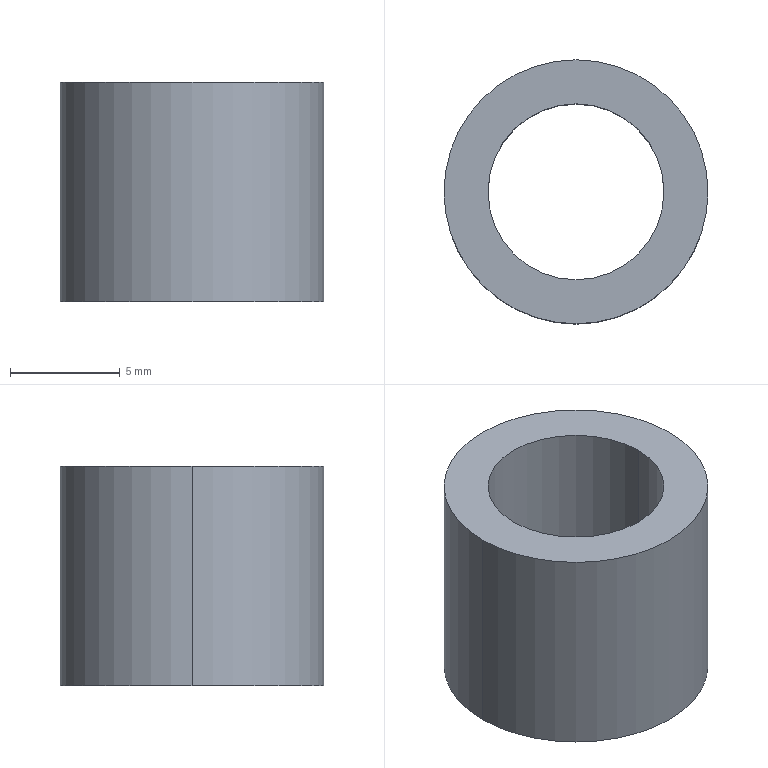Part | SolidWorks | features Extrusion 1 | 1 solid | 6 faces | box 12 x 12 x 10 mm | volume 628.319 mm3 | cylinder 4 | plane 2 | commonest cylinder face diameters 8 x2 12 x2
STEP:
#1=CARTESIAN_POINT('',(-4.,0.,10.));
#2=VERTEX_POINT('',#1);
#3=CARTESIAN_POINT('',(4.,0.,10.));
#4=VERTEX_POINT('',#3);
#5=CARTESIAN_POINT('',(0.,0.,10.));
#6=DIRECTION('',(0.,0.,1.));
#7=DIRECTION('',(1.,0.,0.));
#8=AXIS2_PLACEMENT_3D('',#5,#6,#7);
#9=CIRCLE('',#8,4.);
#10=EDGE_CURVE('',#2,#4,#9,.T.);
#11=ORIENTED_EDGE('',*,*,#10,.T.);
#12=CARTESIAN_POINT('',(4.,0.,0.));
#13=VERTEX_POINT('',#12);
#14=CARTESIAN_POINT('',(4.,0.,10.));
#15=DIRECTION('',(0.,0.,-1.));
#16=VECTOR('',#15,1000.);
#17=LINE('',#14,#16);
#18=EDGE_CURVE('',#4,#13,#17,.T.);
#19=ORIENTED_EDGE('',*,*,#18,.T.);
#20=CARTESIAN_POINT('',(-4.,0.,0.));
#21=VERTEX_POINT('',#20);
#22=CARTESIAN_POINT('',(0.,0.,0.));
#23=DIRECTION('',(0.,0.,1.));
#24=DIRECTION('',(1.,0.,0.));
#25=AXIS2_PLACEMENT_3D('',#22,#23,#24);
#26=CIRCLE('',#25,4.);
#27=EDGE_CURVE('',#21,#13,#26,.T.);
#28=ORIENTED_EDGE('',*,*,#27,.F.);
#29=CARTESIAN_POINT('',(-4.,0.,10.));
#30=DIRECTION('',(0.,0.,-1.));
#31=VECTOR('',#30,1000.);
#32=LINE('',#29,#31);
#33=EDGE_CURVE('',#2,#21,#32,.T.);
#34=ORIENTED_EDGE('',*,*,#33,.F.);
#35=EDGE_LOOP('',(#11,#19,#28,#34));
#36=FACE_OUTER_BOUND('',#35,.T.);
#37=CARTESIAN_POINT('',(0.,0.,10.));
#38=DIRECTION('',(0.,0.,-1.));
#39=DIRECTION('',(-1.,0.,0.));
#40=AXIS2_PLACEMENT_3D('',#37,#38,#39);
#41=CYLINDRICAL_SURFACE('',#40,4.);
#42=ADVANCED_FACE('',(#36),#41,.F.);
#43=CARTESIAN_POINT('',(6.,0.,10.));
#44=VERTEX_POINT('',#43);
#45=CARTESIAN_POINT('',(-6.,0.,10.));
#46=VERTEX_POINT('',#45);
#47=CARTESIAN_POINT('',(0.,0.,10.));
#48=DIRECTION('',(0.,0.,1.));
#49=DIRECTION('',(1.,0.,0.));
#50=AXIS2_PLACEMENT_3D('',#47,#48,#49);
#51=CIRCLE('',#50,6.);
#52=EDGE_CURVE('',#44,#46,#51,.T.);
#53=ORIENTED_EDGE('',*,*,#52,.F.);
#54=CARTESIAN_POINT('',(6.,0.,0.));
#55=VERTEX_POINT('',#54);
#56=CARTESIAN_POINT('',(6.,0.,10.));
#57=DIRECTION('',(0.,0.,-1.));
#58=VECTOR('',#57,1000.);
#59=LINE('',#56,#58);
#60=EDGE_CURVE('',#44,#55,#59,.T.);
#61=ORIENTED_EDGE('',*,*,#60,.T.);
#62=CARTESIAN_POINT('',(-6.,0.,0.));
#63=VERTEX_POINT('',#62);
#64=CARTESIAN_POINT('',(0.,0.,0.));
#65=DIRECTION('',(0.,0.,1.));
#66=DIRECTION('',(1.,0.,0.));
#67=AXIS2_PLACEMENT_3D('',#64,#65,#66);
#68=CIRCLE('',#67,6.);
#69=EDGE_CURVE('',#55,#63,#68,.T.);
#70=ORIENTED_EDGE('',*,*,#69,.T.);
#71=CARTESIAN_POINT('',(-6.,0.,10.));
#72=DIRECTION('',(0.,0.,-1.));
#73=VECTOR('',#72,1000.);
#74=LINE('',#71,#73);
#75=EDGE_CURVE('',#46,#63,#74,.T.);
#76=ORIENTED_EDGE('',*,*,#75,.F.);
#77=EDGE_LOOP('',(#53,#61,#70,#76));
#78=FACE_OUTER_BOUND('',#77,.T.);
#79=CARTESIAN_POINT('',(0.,0.,10.));
#80=DIRECTION('',(0.,0.,-1.));
#81=DIRECTION('',(-1.,0.,0.));
#82=AXIS2_PLACEMENT_3D('',#79,#80,#81);
#83=CYLINDRICAL_SURFACE('',#82,6.);
#84=ADVANCED_FACE('',(#78),#83,.T.);
#85=CARTESIAN_POINT('',(0.,0.,10.));
#86=DIRECTION('',(0.,0.,1.));
#87=DIRECTION('',(1.,0.,0.));
#88=AXIS2_PLACEMENT_3D('',#85,#86,#87);
#89=CIRCLE('',#88,6.);
#90=EDGE_CURVE('',#46,#44,#89,.T.);
#91=ORIENTED_EDGE('',*,*,#90,.T.);
#92=ORIENTED_EDGE('',*,*,#52,.T.);
#93=EDGE_LOOP('',(#91,#92));
#94=FACE_OUTER_BOUND('',#93,.T.);
#95=ORIENTED_EDGE('',*,*,#10,.F.);
#96=CARTESIAN_POINT('',(0.,0.,10.));
#97=DIRECTION('',(0.,0.,1.));
#98=DIRECTION('',(1.,0.,0.));
#99=AXIS2_PLACEMENT_3D('',#96,#97,#98);
#100=CIRCLE('',#99,4.);
#101=EDGE_CURVE('',#4,#2,#100,.T.);
#102=ORIENTED_EDGE('',*,*,#101,.F.);
#103=EDGE_LOOP('',(#95,#102));
#104=FACE_BOUND('',#103,.T.);
#105=CARTESIAN_POINT('',(0.,0.,10.));
#106=DIRECTION('',(0.,0.,1.));
#107=DIRECTION('',(1.,0.,0.));
#108=AXIS2_PLACEMENT_3D('',#105,#106,#107);
#109=PLANE('',#108);
#110=ADVANCED_FACE('',(#94,#104),#109,.T.);
#111=CARTESIAN_POINT('',(0.,0.,0.));
#112=DIRECTION('',(0.,0.,1.));
#113=DIRECTION('',(1.,0.,0.));
#114=AXIS2_PLACEMENT_3D('',#111,#112,#113);
#115=CIRCLE('',#114,6.);
#116=EDGE_CURVE('',#63,#55,#115,.T.);
#117=ORIENTED_EDGE('',*,*,#116,.F.);
#118=ORIENTED_EDGE('',*,*,#69,.F.);
#119=EDGE_LOOP('',(#117,#118));
#120=FACE_OUTER_BOUND('',#119,.T.);
#121=ORIENTED_EDGE('',*,*,#27,.T.);
#122=CARTESIAN_POINT('',(0.,0.,0.));
#123=DIRECTION('',(0.,0.,1.));
#124=DIRECTION('',(1.,0.,0.));
#125=AXIS2_PLACEMENT_3D('',#122,#123,#124);
#126=CIRCLE('',#125,4.);
#127=EDGE_CURVE('',#13,#21,#126,.T.);
#128=ORIENTED_EDGE('',*,*,#127,.T.);
#129=EDGE_LOOP('',(#121,#128));
#130=FACE_BOUND('',#129,.T.);
#131=CARTESIAN_POINT('',(0.,0.,0.));
#132=DIRECTION('',(0.,0.,1.));
#133=DIRECTION('',(1.,0.,0.));
#134=AXIS2_PLACEMENT_3D('',#131,#132,#133);
#135=PLANE('',#134);
#136=ADVANCED_FACE('',(#120,#130),#135,.F.);
#137=ORIENTED_EDGE('',*,*,#60,.F.);
#138=ORIENTED_EDGE('',*,*,#90,.F.);
#139=ORIENTED_EDGE('',*,*,#75,.T.);
#140=ORIENTED_EDGE('',*,*,#116,.T.);
#141=EDGE_LOOP('',(#137,#138,#139,#140));
#142=FACE_OUTER_BOUND('',#141,.T.);
#143=CARTESIAN_POINT('',(0.,0.,10.));
#144=DIRECTION('',(0.,0.,-1.));
#145=DIRECTION('',(-1.,0.,0.));
#146=AXIS2_PLACEMENT_3D('',#143,#144,#145);
#147=CYLINDRICAL_SURFACE('',#146,6.);
#148=ADVANCED_FACE('',(#142),#147,.T.);
#149=ORIENTED_EDGE('',*,*,#18,.F.);
#150=ORIENTED_EDGE('',*,*,#101,.T.);
#151=ORIENTED_EDGE('',*,*,#33,.T.);
#152=ORIENTED_EDGE('',*,*,#127,.F.);
#153=EDGE_LOOP('',(#149,#150,#151,#152));
#154=FACE_OUTER_BOUND('',#153,.T.);
#155=CARTESIAN_POINT('',(0.,0.,10.));
#156=DIRECTION('',(0.,0.,-1.));
#157=DIRECTION('',(-1.,0.,0.));
#158=AXIS2_PLACEMENT_3D('',#155,#156,#157);
#159=CYLINDRICAL_SURFACE('',#158,4.);
#160=ADVANCED_FACE('',(#154),#159,.F.);
#161=CLOSED_SHELL('',(#42,#84,#110,#136,#148,#160));
#162=MANIFOLD_SOLID_BREP('',#161);
#163=CARTESIAN_POINT('',(0.,0.,0.));
#164=DIRECTION('',(0.,0.,1.));
#165=DIRECTION('',(1.,0.,0.));
#166=AXIS2_PLACEMENT_3D('',#163,#164,#165);
#167=(LENGTH_UNIT()NAMED_UNIT(*)SI_UNIT(.MILLI.,.METRE.));
#168=UNCERTAINTY_MEASURE_WITH_UNIT(LENGTH_MEASURE(0.00001),#167,'','');
#169=(NAMED_UNIT(*)PLANE_ANGLE_UNIT()SI_UNIT($,.RADIAN.));
#170=(NAMED_UNIT(*)SI_UNIT($,.STERADIAN.)SOLID_ANGLE_UNIT());
#171=(GEOMETRIC_REPRESENTATION_CONTEXT(3)GLOBAL_UNCERTAINTY_ASSIGNED_CONTEXT((#168))GLOBAL_UNIT_ASSIGNED_CONTEXT((#167,#169,#170))REPRESENTATION_CONTEXT('',''));
#172=ADVANCED_BREP_SHAPE_REPRESENTATION('',(#162,#166),#171);